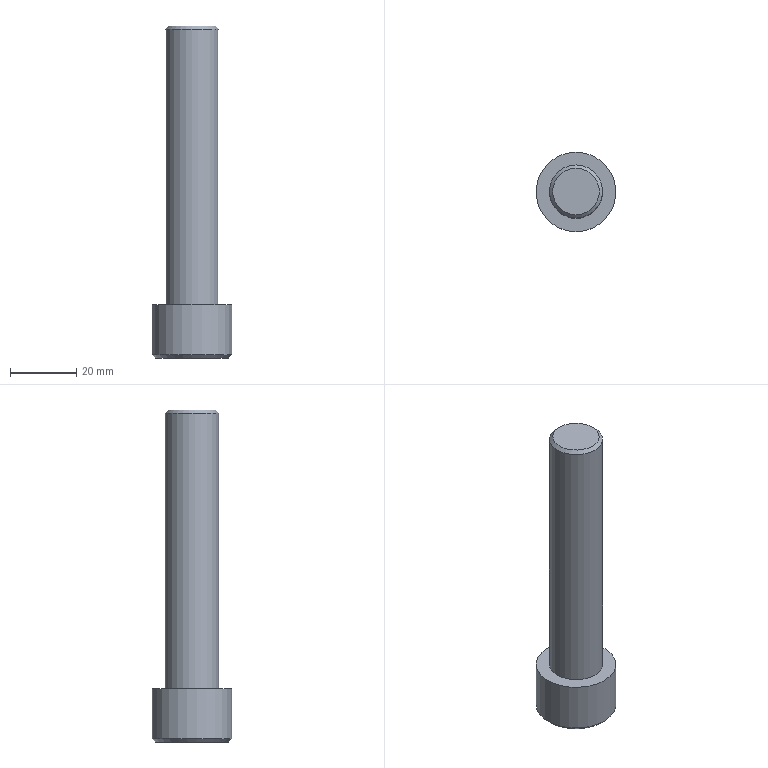Part | STEP file | solid 236 | 1 solid | 14 faces | box 24 x 24 x 100 mm | volume 22879 mm3 | plane 10 | cone 2 | cylinder 2 | commonest cylinder face diameters 16 x1 24 x1